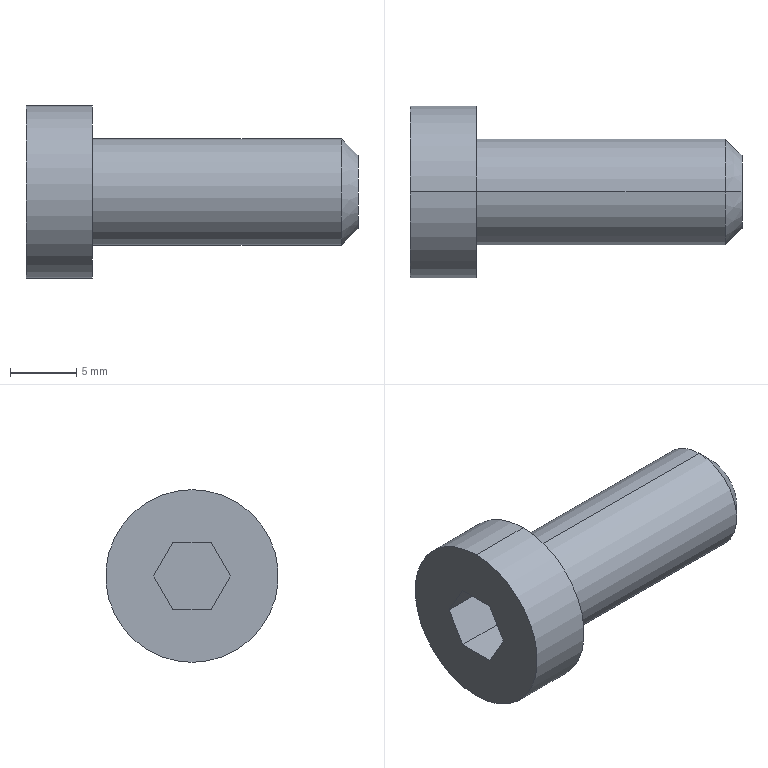Part | STEP file | CBSST8-20 | 1 solid | 16 faces | box 25 x 13 x 13 mm | volume 1569 mm3 | plane 10 | cylinder 4 | cone 2 | commonest cylinder face diameters 8 x2 13 x2
STEP:
#1=CARTESIAN_POINT('',(0.,0.,0.));
#2=DIRECTION('',(0.,0.,1.));
#3=DIRECTION('',(1.,0.,0.));
#4=AXIS2_PLACEMENT_3D('',#1,#2,#3);
#5=CARTESIAN_POINT('',(0.,0.,6.5));
#6=VERTEX_POINT('',#5);
#7=CARTESIAN_POINT('',(0.,0.,-6.5));
#8=VERTEX_POINT('',#7);
#9=CARTESIAN_POINT('',(0.,0.,0.));
#10=DIRECTION('',(-1.,0.,0.));
#11=DIRECTION('',(0.,0.,1.));
#12=AXIS2_PLACEMENT_3D('',#9,#10,#11);
#13=CIRCLE('',#12,6.5);
#14=CARTESIAN_POINT('',(-6.25,0.,0.));
#15=DIRECTION('',(-1.,0.,0.));
#16=DIRECTION('',(0.,0.,1.));
#17=AXIS2_PLACEMENT_3D('',#14,#15,#16);
#18=CYLINDRICAL_SURFACE('',#17,6.5);
#19=CARTESIAN_POINT('',(0.,-6.25));
#20=DIRECTION('',(1.,0.));
#21=VECTOR('',#20,1.);
#22=LINE('',#19,#21);
#23=(GEOMETRIC_REPRESENTATION_CONTEXT(2)PARAMETRIC_REPRESENTATION_CONTEXT()REPRESENTATION_CONTEXT('',''));
#24=DEFINITIONAL_REPRESENTATION('',(#22),#23);
#25=PCURVE('',#18,#24);
#26=CARTESIAN_POINT('',(0.,-4.4,0.));
#27=DIRECTION('',(1.,0.,0.));
#28=DIRECTION('',(0.,0.,-1.));
#29=AXIS2_PLACEMENT_3D('',#26,#27,#28);
#30=PLANE('',#29);
#31=CARTESIAN_POINT('',(-6.5,4.4));
#32=CARTESIAN_POINT('',(-6.5,15.658));
#33=CARTESIAN_POINT('',(3.25,10.029));
#34=CARTESIAN_POINT('',(13.,4.4));
#35=CARTESIAN_POINT('',(3.25,-1.229));
#36=CARTESIAN_POINT('',(-6.5,-6.858));
#37=CARTESIAN_POINT('',(-6.5,4.4));
#38=(BOUNDED_CURVE()B_SPLINE_CURVE(2,(#31,#32,#33,#34,#35,#36,#37),.UNSPECIFIED.,.T.,.F.)B_SPLINE_CURVE_WITH_KNOTS((1,2,2,2,2,1),(-2.094,0.,2.094,4.189,6.283,8.378),.UNSPECIFIED.)CURVE()GEOMETRIC_REPRESENTATION_ITEM()RATIONAL_B_SPLINE_CURVE((1.,0.5,1.,0.5,1.,0.5,1.))REPRESENTATION_ITEM(''));
#39=(GEOMETRIC_REPRESENTATION_CONTEXT(2)PARAMETRIC_REPRESENTATION_CONTEXT()REPRESENTATION_CONTEXT('',''));
#40=DEFINITIONAL_REPRESENTATION('',(#38),#39);
#41=PCURVE('',#30,#40);
#42=SURFACE_CURVE('',#13,(#25,#41),.PCURVE_S1.);
#43=EDGE_CURVE('',#6,#8,#42,.T.);
#44=ORIENTED_EDGE('',*,*,#43,.T.);
#45=CARTESIAN_POINT('',(-5.,0.,-6.5));
#46=VERTEX_POINT('',#45);
#47=CARTESIAN_POINT('',(-6.25,0.,-6.5));
#48=DIRECTION('',(-1.,0.,0.));
#49=VECTOR('',#48,1.);
#50=LINE('',#47,#49);
#51=CARTESIAN_POINT('',(3.142,0.));
#52=DIRECTION('',(0.,1.));
#53=VECTOR('',#52,1.);
#54=LINE('',#51,#53);
#55=(GEOMETRIC_REPRESENTATION_CONTEXT(2)PARAMETRIC_REPRESENTATION_CONTEXT()REPRESENTATION_CONTEXT('',''));
#56=DEFINITIONAL_REPRESENTATION('',(#54),#55);
#57=PCURVE('',#18,#56);
#58=CARTESIAN_POINT('',(-6.25,0.,0.));
#59=DIRECTION('',(-1.,0.,0.));
#60=DIRECTION('',(0.,0.,1.));
#61=AXIS2_PLACEMENT_3D('',#58,#59,#60);
#62=CYLINDRICAL_SURFACE('',#61,6.5);
#63=CARTESIAN_POINT('',(3.142,0.));
#64=DIRECTION('',(0.,1.));
#65=VECTOR('',#64,1.);
#66=LINE('',#63,#65);
#67=(GEOMETRIC_REPRESENTATION_CONTEXT(2)PARAMETRIC_REPRESENTATION_CONTEXT()REPRESENTATION_CONTEXT('',''));
#68=DEFINITIONAL_REPRESENTATION('',(#66),#67);
#69=PCURVE('',#62,#68);
#70=SURFACE_CURVE('',#50,(#57,#69),.PCURVE_S1.);
#71=EDGE_CURVE('',#8,#46,#70,.T.);
#72=ORIENTED_EDGE('',*,*,#71,.T.);
#73=CARTESIAN_POINT('',(-5.,0.,6.5));
#74=VERTEX_POINT('',#73);
#75=CARTESIAN_POINT('',(-5.,0.,0.));
#76=DIRECTION('',(-1.,0.,0.));
#77=DIRECTION('',(0.,0.,1.));
#78=AXIS2_PLACEMENT_3D('',#75,#76,#77);
#79=CIRCLE('',#78,6.5);
#80=CARTESIAN_POINT('',(0.,-1.25));
#81=DIRECTION('',(1.,0.));
#82=VECTOR('',#81,1.);
#83=LINE('',#80,#82);
#84=(GEOMETRIC_REPRESENTATION_CONTEXT(2)PARAMETRIC_REPRESENTATION_CONTEXT()REPRESENTATION_CONTEXT('',''));
#85=DEFINITIONAL_REPRESENTATION('',(#83),#84);
#86=PCURVE('',#18,#85);
#87=CARTESIAN_POINT('',(-5.,-6.5,0.));
#88=DIRECTION('',(-1.,0.,0.));
#89=DIRECTION('',(0.,0.,1.));
#90=AXIS2_PLACEMENT_3D('',#87,#88,#89);
#91=PLANE('',#90);
#92=CARTESIAN_POINT('',(0.,6.5));
#93=DIRECTION('',(1.,0.));
#94=AXIS2_PLACEMENT_2D('',#92,#93);
#95=CIRCLE('',#94,6.5);
#96=(GEOMETRIC_REPRESENTATION_CONTEXT(2)PARAMETRIC_REPRESENTATION_CONTEXT()REPRESENTATION_CONTEXT('',''));
#97=DEFINITIONAL_REPRESENTATION('',(#95),#96);
#98=PCURVE('',#91,#97);
#99=SURFACE_CURVE('',#79,(#86,#98),.PCURVE_S1.);
#100=EDGE_CURVE('',#74,#46,#99,.T.);
#101=ORIENTED_EDGE('',*,*,#100,.F.);
#102=CARTESIAN_POINT('',(-6.25,0.,6.5));
#103=DIRECTION('',(-1.,0.,0.));
#104=VECTOR('',#103,1.);
#105=LINE('',#102,#104);
#106=CARTESIAN_POINT('',(0.,0.));
#107=DIRECTION('',(0.,1.));
#108=VECTOR('',#107,1.);
#109=LINE('',#106,#108);
#110=(GEOMETRIC_REPRESENTATION_CONTEXT(2)PARAMETRIC_REPRESENTATION_CONTEXT()REPRESENTATION_CONTEXT('',''));
#111=DEFINITIONAL_REPRESENTATION('',(#109),#110);
#112=PCURVE('',#18,#111);
#113=CARTESIAN_POINT('',(6.283,0.));
#114=DIRECTION('',(0.,1.));
#115=VECTOR('',#114,1.);
#116=LINE('',#113,#115);
#117=(GEOMETRIC_REPRESENTATION_CONTEXT(2)PARAMETRIC_REPRESENTATION_CONTEXT()REPRESENTATION_CONTEXT('',''));
#118=DEFINITIONAL_REPRESENTATION('',(#116),#117);
#119=PCURVE('',#62,#118);
#120=SURFACE_CURVE('',#105,(#112,#119),.PCURVE_S1.);
#121=EDGE_CURVE('',#6,#74,#120,.T.);
#122=ORIENTED_EDGE('',*,*,#121,.F.);
#123=EDGE_LOOP('',(#44,#72,#101,#122));
#124=FACE_BOUND('',#123,.T.);
#125=ADVANCED_FACE('',(#124),#18,.T.);
#126=CARTESIAN_POINT('',(18.75,0.,4.));
#127=VERTEX_POINT('',#126);
#128=CARTESIAN_POINT('',(18.75,0.,-4.));
#129=VERTEX_POINT('',#128);
#130=CARTESIAN_POINT('',(18.75,0.,0.));
#131=DIRECTION('',(-1.,0.,0.));
#132=DIRECTION('',(0.,0.,1.));
#133=AXIS2_PLACEMENT_3D('',#130,#131,#132);
#134=CIRCLE('',#133,4.);
#135=CARTESIAN_POINT('',(-6.25,0.,0.));
#136=DIRECTION('',(-1.,0.,0.));
#137=DIRECTION('',(0.,0.,1.));
#138=AXIS2_PLACEMENT_3D('',#135,#136,#137);
#139=CYLINDRICAL_SURFACE('',#138,4.);
#140=CARTESIAN_POINT('',(0.,-25.));
#141=DIRECTION('',(1.,0.));
#142=VECTOR('',#141,1.);
#143=LINE('',#140,#142);
#144=(GEOMETRIC_REPRESENTATION_CONTEXT(2)PARAMETRIC_REPRESENTATION_CONTEXT()REPRESENTATION_CONTEXT('',''));
#145=DEFINITIONAL_REPRESENTATION('',(#143),#144);
#146=PCURVE('',#139,#145);
#147=CARTESIAN_POINT('',(18.75,0.,0.));
#148=DIRECTION('',(-1.,0.,0.));
#149=DIRECTION('',(0.,0.,1.));
#150=AXIS2_PLACEMENT_3D('',#147,#148,#149);
#151=CONICAL_SURFACE('',#150,4.,0.7854);
#152=CARTESIAN_POINT('',(0.,0.));
#153=DIRECTION('',(1.,0.));
#154=VECTOR('',#153,1.);
#155=LINE('',#152,#154);
#156=(GEOMETRIC_REPRESENTATION_CONTEXT(2)PARAMETRIC_REPRESENTATION_CONTEXT()REPRESENTATION_CONTEXT('',''));
#157=DEFINITIONAL_REPRESENTATION('',(#155),#156);
#158=PCURVE('',#151,#157);
#159=SURFACE_CURVE('',#134,(#146,#158),.PCURVE_S1.);
#160=EDGE_CURVE('',#127,#129,#159,.T.);
#161=ORIENTED_EDGE('',*,*,#160,.T.);
#162=CARTESIAN_POINT('',(0.,0.,-4.));
#163=VERTEX_POINT('',#162);
#164=CARTESIAN_POINT('',(-6.25,0.,-4.));
#165=DIRECTION('',(-1.,0.,0.));
#166=VECTOR('',#165,1.);
#167=LINE('',#164,#166);
#168=CARTESIAN_POINT('',(3.142,0.));
#169=DIRECTION('',(0.,1.));
#170=VECTOR('',#169,1.);
#171=LINE('',#168,#170);
#172=(GEOMETRIC_REPRESENTATION_CONTEXT(2)PARAMETRIC_REPRESENTATION_CONTEXT()REPRESENTATION_CONTEXT('',''));
#173=DEFINITIONAL_REPRESENTATION('',(#171),#172);
#174=PCURVE('',#139,#173);
#175=CARTESIAN_POINT('',(-6.25,0.,0.));
#176=DIRECTION('',(-1.,0.,0.));
#177=DIRECTION('',(0.,0.,1.));
#178=AXIS2_PLACEMENT_3D('',#175,#176,#177);
#179=CYLINDRICAL_SURFACE('',#178,4.);
#180=CARTESIAN_POINT('',(3.142,0.));
#181=DIRECTION('',(0.,1.));
#182=VECTOR('',#181,1.);
#183=LINE('',#180,#182);
#184=(GEOMETRIC_REPRESENTATION_CONTEXT(2)PARAMETRIC_REPRESENTATION_CONTEXT()REPRESENTATION_CONTEXT('',''));
#185=DEFINITIONAL_REPRESENTATION('',(#183),#184);
#186=PCURVE('',#179,#185);
#187=SURFACE_CURVE('',#167,(#174,#186),.PCURVE_S1.);
#188=EDGE_CURVE('',#129,#163,#187,.T.);
#189=ORIENTED_EDGE('',*,*,#188,.T.);
#190=CARTESIAN_POINT('',(0.,0.,4.));
#191=VERTEX_POINT('',#190);
#192=CARTESIAN_POINT('',(0.,0.,0.));
#193=DIRECTION('',(1.,0.,0.));
#194=DIRECTION('',(0.,0.,-1.));
#195=AXIS2_PLACEMENT_3D('',#192,#193,#194);
#196=CIRCLE('',#195,4.);
#197=CARTESIAN_POINT('',(3.142,-6.25));
#198=DIRECTION('',(-1.,0.));
#199=VECTOR('',#198,1.);
#200=LINE('',#197,#199);
#201=(GEOMETRIC_REPRESENTATION_CONTEXT(2)PARAMETRIC_REPRESENTATION_CONTEXT()REPRESENTATION_CONTEXT('',''));
#202=DEFINITIONAL_REPRESENTATION('',(#200),#201);
#203=PCURVE('',#139,#202);
#204=CARTESIAN_POINT('',(0.,4.4));
#205=DIRECTION('',(1.,0.));
#206=AXIS2_PLACEMENT_2D('',#204,#205);
#207=CIRCLE('',#206,4.);
#208=(GEOMETRIC_REPRESENTATION_CONTEXT(2)PARAMETRIC_REPRESENTATION_CONTEXT()REPRESENTATION_CONTEXT('',''));
#209=DEFINITIONAL_REPRESENTATION('',(#207),#208);
#210=PCURVE('',#30,#209);
#211=SURFACE_CURVE('',#196,(#203,#210),.PCURVE_S1.);
#212=EDGE_CURVE('',#163,#191,#211,.T.);
#213=ORIENTED_EDGE('',*,*,#212,.T.);
#214=CARTESIAN_POINT('',(-6.25,0.,4.));
#215=DIRECTION('',(-1.,0.,0.));
#216=VECTOR('',#215,1.);
#217=LINE('',#214,#216);
#218=CARTESIAN_POINT('',(0.,0.));
#219=DIRECTION('',(0.,1.));
#220=VECTOR('',#219,1.);
#221=LINE('',#218,#220);
#222=(GEOMETRIC_REPRESENTATION_CONTEXT(2)PARAMETRIC_REPRESENTATION_CONTEXT()REPRESENTATION_CONTEXT('',''));
#223=DEFINITIONAL_REPRESENTATION('',(#221),#222);
#224=PCURVE('',#139,#223);
#225=CARTESIAN_POINT('',(6.283,0.));
#226=DIRECTION('',(0.,1.));
#227=VECTOR('',#226,1.);
#228=LINE('',#225,#227);
#229=(GEOMETRIC_REPRESENTATION_CONTEXT(2)PARAMETRIC_REPRESENTATION_CONTEXT()REPRESENTATION_CONTEXT('',''));
#230=DEFINITIONAL_REPRESENTATION('',(#228),#229);
#231=PCURVE('',#179,#230);
#232=SURFACE_CURVE('',#217,(#224,#231),.PCURVE_S1.);
#233=EDGE_CURVE('',#127,#191,#232,.T.);
#234=ORIENTED_EDGE('',*,*,#233,.F.);
#235=EDGE_LOOP('',(#161,#189,#213,#234));
#236=FACE_BOUND('',#235,.T.);
#237=ADVANCED_FACE('',(#236),#139,.T.);
#238=CARTESIAN_POINT('',(20.,0.,2.75));
#239=VERTEX_POINT('',#238);
#240=CARTESIAN_POINT('',(20.,0.,-2.75));
#241=VERTEX_POINT('',#240);
#242=CARTESIAN_POINT('',(20.,0.,0.));
#243=DIRECTION('',(-1.,0.,0.));
#244=DIRECTION('',(0.,0.,1.));
#245=AXIS2_PLACEMENT_3D('',#242,#243,#244);
#246=CIRCLE('',#245,2.75);
#247=CARTESIAN_POINT('',(0.,-1.25));
#248=DIRECTION('',(1.,0.));
#249=VECTOR('',#248,1.);
#250=LINE('',#247,#249);
#251=(GEOMETRIC_REPRESENTATION_CONTEXT(2)PARAMETRIC_REPRESENTATION_CONTEXT()REPRESENTATION_CONTEXT('',''));
#252=DEFINITIONAL_REPRESENTATION('',(#250),#251);
#253=PCURVE('',#151,#252);
#254=CARTESIAN_POINT('',(20.,0.,0.));
#255=DIRECTION('',(1.,0.,0.));
#256=DIRECTION('',(0.,0.,-1.));
#257=AXIS2_PLACEMENT_3D('',#254,#255,#256);
#258=PLANE('',#257);
#259=CARTESIAN_POINT('',(-2.75,0.));
#260=CARTESIAN_POINT('',(-2.75,4.763));
#261=CARTESIAN_POINT('',(1.375,2.382));
#262=CARTESIAN_POINT('',(5.5,0.));
#263=CARTESIAN_POINT('',(1.375,-2.382));
#264=CARTESIAN_POINT('',(-2.75,-4.763));
#265=CARTESIAN_POINT('',(-2.75,0.));
#266=(BOUNDED_CURVE()B_SPLINE_CURVE(2,(#259,#260,#261,#262,#263,#264,#265),.UNSPECIFIED.,.T.,.F.)B_SPLINE_CURVE_WITH_KNOTS((1,2,2,2,2,1),(-2.094,0.,2.094,4.189,6.283,8.378),.UNSPECIFIED.)CURVE()GEOMETRIC_REPRESENTATION_ITEM()RATIONAL_B_SPLINE_CURVE((1.,0.5,1.,0.5,1.,0.5,1.))REPRESENTATION_ITEM(''));
#267=(GEOMETRIC_REPRESENTATION_CONTEXT(2)PARAMETRIC_REPRESENTATION_CONTEXT()REPRESENTATION_CONTEXT('',''));
#268=DEFINITIONAL_REPRESENTATION('',(#266),#267);
#269=PCURVE('',#258,#268);
#270=SURFACE_CURVE('',#246,(#253,#269),.PCURVE_S1.);
#271=EDGE_CURVE('',#239,#241,#270,.T.);
#272=ORIENTED_EDGE('',*,*,#271,.T.);
#273=CARTESIAN_POINT('',(18.75,0.,-4.));
#274=DIRECTION('',(-0.7071,0.,-0.7071));
#275=VECTOR('',#274,1.);
#276=LINE('',#273,#275);
#277=CARTESIAN_POINT('',(3.142,0.));
#278=DIRECTION('',(0.,1.));
#279=VECTOR('',#278,1.);
#280=LINE('',#277,#279);
#281=(GEOMETRIC_REPRESENTATION_CONTEXT(2)PARAMETRIC_REPRESENTATION_CONTEXT()REPRESENTATION_CONTEXT('',''));
#282=DEFINITIONAL_REPRESENTATION('',(#280),#281);
#283=PCURVE('',#151,#282);
#284=CARTESIAN_POINT('',(18.75,0.,0.));
#285=DIRECTION('',(-1.,0.,0.));
#286=DIRECTION('',(0.,0.,1.));
#287=AXIS2_PLACEMENT_3D('',#284,#285,#286);
#288=CONICAL_SURFACE('',#287,4.,0.7854);
#289=CARTESIAN_POINT('',(3.142,0.));
#290=DIRECTION('',(0.,1.));
#291=VECTOR('',#290,1.);
#292=LINE('',#289,#291);
#293=(GEOMETRIC_REPRESENTATION_CONTEXT(2)PARAMETRIC_REPRESENTATION_CONTEXT()REPRESENTATION_CONTEXT('',''));
#294=DEFINITIONAL_REPRESENTATION('',(#292),#293);
#295=PCURVE('',#288,#294);
#296=SURFACE_CURVE('',#276,(#283,#295),.PCURVE_S1.);
#297=EDGE_CURVE('',#241,#129,#296,.T.);
#298=ORIENTED_EDGE('',*,*,#297,.T.);
#299=ORIENTED_EDGE('',*,*,#160,.F.);
#300=CARTESIAN_POINT('',(18.75,0.,4.));
#301=DIRECTION('',(-0.7071,0.,0.7071));
#302=VECTOR('',#301,1.);
#303=LINE('',#300,#302);
#304=CARTESIAN_POINT('',(0.,0.));
#305=DIRECTION('',(0.,1.));
#306=VECTOR('',#305,1.);
#307=LINE('',#304,#306);
#308=(GEOMETRIC_REPRESENTATION_CONTEXT(2)PARAMETRIC_REPRESENTATION_CONTEXT()REPRESENTATION_CONTEXT('',''));
#309=DEFINITIONAL_REPRESENTATION('',(#307),#308);
#310=PCURVE('',#151,#309);
#311=CARTESIAN_POINT('',(6.283,0.));
#312=DIRECTION('',(0.,1.));
#313=VECTOR('',#312,1.);
#314=LINE('',#311,#313);
#315=(GEOMETRIC_REPRESENTATION_CONTEXT(2)PARAMETRIC_REPRESENTATION_CONTEXT()REPRESENTATION_CONTEXT('',''));
#316=DEFINITIONAL_REPRESENTATION('',(#314),#315);
#317=PCURVE('',#288,#316);
#318=SURFACE_CURVE('',#303,(#310,#317),.PCURVE_S1.);
#319=EDGE_CURVE('',#239,#127,#318,.T.);
#320=ORIENTED_EDGE('',*,*,#319,.F.);
#321=EDGE_LOOP('',(#272,#298,#299,#320));
#322=FACE_BOUND('',#321,.T.);
#323=ADVANCED_FACE('',(#322),#151,.T.);
#324=CARTESIAN_POINT('',(-5.,1.443,2.5));
#325=VERTEX_POINT('',#324);
#326=CARTESIAN_POINT('',(-5.,2.887,0.));
#327=VERTEX_POINT('',#326);
#328=CARTESIAN_POINT('',(-5.,1.443,2.5));
#329=DIRECTION('',(0.,0.5,-0.866));
#330=VECTOR('',#329,1.);
#331=LINE('',#328,#330);
#332=CARTESIAN_POINT('',(2.5,7.943));
#333=DIRECTION('',(-0.866,0.5));
#334=VECTOR('',#333,1.);
#335=LINE('',#332,#334);
#336=(GEOMETRIC_REPRESENTATION_CONTEXT(2)PARAMETRIC_REPRESENTATION_CONTEXT()REPRESENTATION_CONTEXT('',''));
#337=DEFINITIONAL_REPRESENTATION('',(#335),#336);
#338=PCURVE('',#91,#337);
#339=CARTESIAN_POINT('',(-1.2,1.443,2.5));
#340=DIRECTION('',(0.,0.866,0.5));
#341=DIRECTION('',(0.,-0.5,0.866));
#342=AXIS2_PLACEMENT_3D('',#339,#340,#341);
#343=PLANE('',#342);
#344=CARTESIAN_POINT('',(0.,-3.8));
#345=DIRECTION('',(-1.,0.));
#346=VECTOR('',#345,1.);
#347=LINE('',#344,#346);
#348=(GEOMETRIC_REPRESENTATION_CONTEXT(2)PARAMETRIC_REPRESENTATION_CONTEXT()REPRESENTATION_CONTEXT('',''));
#349=DEFINITIONAL_REPRESENTATION('',(#347),#348);
#350=PCURVE('',#343,#349);
#351=SURFACE_CURVE('',#331,(#338,#350),.PCURVE_S1.);
#352=EDGE_CURVE('',#325,#327,#351,.T.);
#353=ORIENTED_EDGE('',*,*,#352,.F.);
#354=CARTESIAN_POINT('',(-5.,-1.443,2.5));
#355=VERTEX_POINT('',#354);
#356=CARTESIAN_POINT('',(-5.,-1.443,2.5));
#357=DIRECTION('',(0.,1.,0.));
#358=VECTOR('',#357,1.);
#359=LINE('',#356,#358);
#360=CARTESIAN_POINT('',(2.5,5.057));
#361=DIRECTION('',(0.,1.));
#362=VECTOR('',#361,1.);
#363=LINE('',#360,#362);
#364=(GEOMETRIC_REPRESENTATION_CONTEXT(2)PARAMETRIC_REPRESENTATION_CONTEXT()REPRESENTATION_CONTEXT('',''));
#365=DEFINITIONAL_REPRESENTATION('',(#363),#364);
#366=PCURVE('',#91,#365);
#367=CARTESIAN_POINT('',(-1.2,-1.443,2.5));
#368=DIRECTION('',(0.,0.,1.));
#369=DIRECTION('',(1.,0.,0.));
#370=AXIS2_PLACEMENT_3D('',#367,#368,#369);
#371=PLANE('',#370);
#372=CARTESIAN_POINT('',(-3.8,0.));
#373=DIRECTION('',(0.,1.));
#374=VECTOR('',#373,1.);
#375=LINE('',#372,#374);
#376=(GEOMETRIC_REPRESENTATION_CONTEXT(2)PARAMETRIC_REPRESENTATION_CONTEXT()REPRESENTATION_CONTEXT('',''));
#377=DEFINITIONAL_REPRESENTATION('',(#375),#376);
#378=PCURVE('',#371,#377);
#379=SURFACE_CURVE('',#359,(#366,#378),.PCURVE_S1.);
#380=EDGE_CURVE('',#355,#325,#379,.T.);
#381=ORIENTED_EDGE('',*,*,#380,.F.);
#382=CARTESIAN_POINT('',(-5.,-2.887,0.));
#383=VERTEX_POINT('',#382);
#384=CARTESIAN_POINT('',(-5.,-2.887,0.));
#385=DIRECTION('',(0.,0.5,0.866));
#386=VECTOR('',#385,1.);
#387=LINE('',#384,#386);
#388=CARTESIAN_POINT('',(0.,3.613));
#389=DIRECTION('',(0.866,0.5));
#390=VECTOR('',#389,1.);
#391=LINE('',#388,#390);
#392=(GEOMETRIC_REPRESENTATION_CONTEXT(2)PARAMETRIC_REPRESENTATION_CONTEXT()REPRESENTATION_CONTEXT('',''));
#393=DEFINITIONAL_REPRESENTATION('',(#391),#392);
#394=PCURVE('',#91,#393);
#395=CARTESIAN_POINT('',(-1.2,-2.887,0.));
#396=DIRECTION('',(0.,-0.866,0.5));
#397=DIRECTION('',(0.,-0.5,-0.866));
#398=AXIS2_PLACEMENT_3D('',#395,#396,#397);
#399=PLANE('',#398);
#400=CARTESIAN_POINT('',(0.,-3.8));
#401=DIRECTION('',(-1.,0.));
#402=VECTOR('',#401,1.);
#403=LINE('',#400,#402);
#404=(GEOMETRIC_REPRESENTATION_CONTEXT(2)PARAMETRIC_REPRESENTATION_CONTEXT()REPRESENTATION_CONTEXT('',''));
#405=DEFINITIONAL_REPRESENTATION('',(#403),#404);
#406=PCURVE('',#399,#405);
#407=SURFACE_CURVE('',#387,(#394,#406),.PCURVE_S1.);
#408=EDGE_CURVE('',#383,#355,#407,.T.);
#409=ORIENTED_EDGE('',*,*,#408,.F.);
#410=CARTESIAN_POINT('',(-5.,-1.443,-2.5));
#411=VERTEX_POINT('',#410);
#412=CARTESIAN_POINT('',(-5.,-1.443,-2.5));
#413=DIRECTION('',(0.,-0.5,0.866));
#414=VECTOR('',#413,1.);
#415=LINE('',#412,#414);
#416=CARTESIAN_POINT('',(-2.5,5.057));
#417=DIRECTION('',(0.866,-0.5));
#418=VECTOR('',#417,1.);
#419=LINE('',#416,#418);
#420=(GEOMETRIC_REPRESENTATION_CONTEXT(2)PARAMETRIC_REPRESENTATION_CONTEXT()REPRESENTATION_CONTEXT('',''));
#421=DEFINITIONAL_REPRESENTATION('',(#419),#420);
#422=PCURVE('',#91,#421);
#423=CARTESIAN_POINT('',(-1.2,-1.443,-2.5));
#424=DIRECTION('',(0.,-0.866,-0.5));
#425=DIRECTION('',(0.,0.5,-0.866));
#426=AXIS2_PLACEMENT_3D('',#423,#424,#425);
#427=PLANE('',#426);
#428=CARTESIAN_POINT('',(0.,-3.8));
#429=DIRECTION('',(-1.,0.));
#430=VECTOR('',#429,1.);
#431=LINE('',#428,#430);
#432=(GEOMETRIC_REPRESENTATION_CONTEXT(2)PARAMETRIC_REPRESENTATION_CONTEXT()REPRESENTATION_CONTEXT('',''));
#433=DEFINITIONAL_REPRESENTATION('',(#431),#432);
#434=PCURVE('',#427,#433);
#435=SURFACE_CURVE('',#415,(#422,#434),.PCURVE_S1.);
#436=EDGE_CURVE('',#411,#383,#435,.T.);
#437=ORIENTED_EDGE('',*,*,#436,.F.);
#438=CARTESIAN_POINT('',(-5.,1.443,-2.5));
#439=VERTEX_POINT('',#438);
#440=CARTESIAN_POINT('',(-5.,1.443,-2.5));
#441=DIRECTION('',(0.,-1.,0.));
#442=VECTOR('',#441,1.);
#443=LINE('',#440,#442);
#444=CARTESIAN_POINT('',(-2.5,7.943));
#445=DIRECTION('',(0.,-1.));
#446=VECTOR('',#445,1.);
#447=LINE('',#444,#446);
#448=(GEOMETRIC_REPRESENTATION_CONTEXT(2)PARAMETRIC_REPRESENTATION_CONTEXT()REPRESENTATION_CONTEXT('',''));
#449=DEFINITIONAL_REPRESENTATION('',(#447),#448);
#450=PCURVE('',#91,#449);
#451=CARTESIAN_POINT('',(-1.2,1.443,-2.5));
#452=DIRECTION('',(0.,0.,-1.));
#453=DIRECTION('',(-1.,0.,0.));
#454=AXIS2_PLACEMENT_3D('',#451,#452,#453);
#455=PLANE('',#454);
#456=CARTESIAN_POINT('',(3.8,0.));
#457=DIRECTION('',(0.,-1.));
#458=VECTOR('',#457,1.);
#459=LINE('',#456,#458);
#460=(GEOMETRIC_REPRESENTATION_CONTEXT(2)PARAMETRIC_REPRESENTATION_CONTEXT()REPRESENTATION_CONTEXT('',''));
#461=DEFINITIONAL_REPRESENTATION('',(#459),#460);
#462=PCURVE('',#455,#461);
#463=SURFACE_CURVE('',#443,(#450,#462),.PCURVE_S1.);
#464=EDGE_CURVE('',#439,#411,#463,.T.);
#465=ORIENTED_EDGE('',*,*,#464,.F.);
#466=CARTESIAN_POINT('',(-5.,2.887,0.));
#467=DIRECTION('',(0.,-0.5,-0.866));
#468=VECTOR('',#467,1.);
#469=LINE('',#466,#468);
#470=CARTESIAN_POINT('',(0.,9.387));
#471=DIRECTION('',(-0.866,-0.5));
#472=VECTOR('',#471,1.);
#473=LINE('',#470,#472);
#474=(GEOMETRIC_REPRESENTATION_CONTEXT(2)PARAMETRIC_REPRESENTATION_CONTEXT()REPRESENTATION_CONTEXT('',''));
#475=DEFINITIONAL_REPRESENTATION('',(#473),#474);
#476=PCURVE('',#91,#475);
#477=CARTESIAN_POINT('',(-1.2,2.887,0.));
#478=DIRECTION('',(0.,0.866,-0.5));
#479=DIRECTION('',(0.,0.5,0.866));
#480=AXIS2_PLACEMENT_3D('',#477,#478,#479);
#481=PLANE('',#480);
#482=CARTESIAN_POINT('',(0.,-3.8));
#483=DIRECTION('',(-1.,0.));
#484=VECTOR('',#483,1.);
#485=LINE('',#482,#484);
#486=(GEOMETRIC_REPRESENTATION_CONTEXT(2)PARAMETRIC_REPRESENTATION_CONTEXT()REPRESENTATION_CONTEXT('',''));
#487=DEFINITIONAL_REPRESENTATION('',(#485),#486);
#488=PCURVE('',#481,#487);
#489=SURFACE_CURVE('',#469,(#476,#488),.PCURVE_S1.);
#490=EDGE_CURVE('',#327,#439,#489,.T.);
#491=ORIENTED_EDGE('',*,*,#490,.F.);
#492=EDGE_LOOP('',(#353,#381,#409,#437,#465,#491));
#493=FACE_BOUND('',#492,.T.);
#494=ORIENTED_EDGE('',*,*,#100,.T.);
#495=CARTESIAN_POINT('',(-5.,0.,0.));
#496=DIRECTION('',(-1.,0.,0.));
#497=DIRECTION('',(0.,0.,1.));
#498=AXIS2_PLACEMENT_3D('',#495,#496,#497);
#499=CIRCLE('',#498,6.5);
#500=CARTESIAN_POINT('',(0.,6.5));
#501=DIRECTION('',(1.,0.));
#502=AXIS2_PLACEMENT_2D('',#500,#501);
#503=CIRCLE('',#502,6.5);
#504=(GEOMETRIC_REPRESENTATION_CONTEXT(2)PARAMETRIC_REPRESENTATION_CONTEXT()REPRESENTATION_CONTEXT('',''));
#505=DEFINITIONAL_REPRESENTATION('',(#503),#504);
#506=PCURVE('',#91,#505);
#507=CARTESIAN_POINT('',(0.,-1.25));
#508=DIRECTION('',(1.,0.));
#509=VECTOR('',#508,1.);
#510=LINE('',#507,#509);
#511=(GEOMETRIC_REPRESENTATION_CONTEXT(2)PARAMETRIC_REPRESENTATION_CONTEXT()REPRESENTATION_CONTEXT('',''));
#512=DEFINITIONAL_REPRESENTATION('',(#510),#511);
#513=PCURVE('',#62,#512);
#514=SURFACE_CURVE('',#499,(#506,#513),.PCURVE_S1.);
#515=EDGE_CURVE('',#46,#74,#514,.T.);
#516=ORIENTED_EDGE('',*,*,#515,.T.);
#517=EDGE_LOOP('',(#494,#516));
#518=FACE_BOUND('',#517,.T.);
#519=ADVANCED_FACE('',(#493,#518),#91,.T.);
#520=ORIENTED_EDGE('',*,*,#271,.F.);
#521=CARTESIAN_POINT('',(20.,0.,0.));
#522=DIRECTION('',(-1.,0.,0.));
#523=DIRECTION('',(0.,0.,1.));
#524=AXIS2_PLACEMENT_3D('',#521,#522,#523);
#525=CIRCLE('',#524,2.75);
#526=CARTESIAN_POINT('',(-2.75,0.));
#527=CARTESIAN_POINT('',(-2.75,4.763));
#528=CARTESIAN_POINT('',(1.375,2.382));
#529=CARTESIAN_POINT('',(5.5,0.));
#530=CARTESIAN_POINT('',(1.375,-2.382));
#531=CARTESIAN_POINT('',(-2.75,-4.763));
#532=CARTESIAN_POINT('',(-2.75,0.));
#533=(BOUNDED_CURVE()B_SPLINE_CURVE(2,(#526,#527,#528,#529,#530,#531,#532),.UNSPECIFIED.,.T.,.F.)B_SPLINE_CURVE_WITH_KNOTS((1,2,2,2,2,1),(-2.094,0.,2.094,4.189,6.283,8.378),.UNSPECIFIED.)CURVE()GEOMETRIC_REPRESENTATION_ITEM()RATIONAL_B_SPLINE_CURVE((1.,0.5,1.,0.5,1.,0.5,1.))REPRESENTATION_ITEM(''));
#534=(GEOMETRIC_REPRESENTATION_CONTEXT(2)PARAMETRIC_REPRESENTATION_CONTEXT()REPRESENTATION_CONTEXT('',''));
#535=DEFINITIONAL_REPRESENTATION('',(#533),#534);
#536=PCURVE('',#258,#535);
#537=CARTESIAN_POINT('',(0.,-1.25));
#538=DIRECTION('',(1.,0.));
#539=VECTOR('',#538,1.);
#540=LINE('',#537,#539);
#541=(GEOMETRIC_REPRESENTATION_CONTEXT(2)PARAMETRIC_REPRESENTATION_CONTEXT()REPRESENTATION_CONTEXT('',''));
#542=DEFINITIONAL_REPRESENTATION('',(#540),#541);
#543=PCURVE('',#288,#542);
#544=SURFACE_CURVE('',#525,(#536,#543),.PCURVE_S1.);
#545=EDGE_CURVE('',#241,#239,#544,.T.);
#546=ORIENTED_EDGE('',*,*,#545,.F.);
#547=EDGE_LOOP('',(#520,#546));
#548=FACE_BOUND('',#547,.T.);
#549=ADVANCED_FACE('',(#548),#258,.T.);
#550=ORIENTED_EDGE('',*,*,#297,.F.);
#551=ORIENTED_EDGE('',*,*,#545,.T.);
#552=ORIENTED_EDGE('',*,*,#319,.T.);
#553=CARTESIAN_POINT('',(18.75,0.,0.));
#554=DIRECTION('',(-1.,0.,0.));
#555=DIRECTION('',(0.,0.,1.));
#556=AXIS2_PLACEMENT_3D('',#553,#554,#555);
#557=CIRCLE('',#556,4.);
#558=CARTESIAN_POINT('',(0.,0.));
#559=DIRECTION('',(1.,0.));
#560=VECTOR('',#559,1.);
#561=LINE('',#558,#560);
#562=(GEOMETRIC_REPRESENTATION_CONTEXT(2)PARAMETRIC_REPRESENTATION_CONTEXT()REPRESENTATION_CONTEXT('',''));
#563=DEFINITIONAL_REPRESENTATION('',(#561),#562);
#564=PCURVE('',#288,#563);
#565=CARTESIAN_POINT('',(0.,-25.));
#566=DIRECTION('',(1.,0.));
#567=VECTOR('',#566,1.);
#568=LINE('',#565,#567);
#569=(GEOMETRIC_REPRESENTATION_CONTEXT(2)PARAMETRIC_REPRESENTATION_CONTEXT()REPRESENTATION_CONTEXT('',''));
#570=DEFINITIONAL_REPRESENTATION('',(#568),#569);
#571=PCURVE('',#179,#570);
#572=SURFACE_CURVE('',#557,(#564,#571),.PCURVE_S1.);
#573=EDGE_CURVE('',#129,#127,#572,.T.);
#574=ORIENTED_EDGE('',*,*,#573,.F.);
#575=EDGE_LOOP('',(#550,#551,#552,#574));
#576=FACE_BOUND('',#575,.T.);
#577=ADVANCED_FACE('',(#576),#288,.T.);
#578=ORIENTED_EDGE('',*,*,#188,.F.);
#579=ORIENTED_EDGE('',*,*,#573,.T.);
#580=ORIENTED_EDGE('',*,*,#233,.T.);
#581=CARTESIAN_POINT('',(0.,0.,0.));
#582=DIRECTION('',(1.,0.,0.));
#583=DIRECTION('',(0.,0.,-1.));
#584=AXIS2_PLACEMENT_3D('',#581,#582,#583);
#585=CIRCLE('',#584,4.);
#586=CARTESIAN_POINT('',(9.425,-6.25));
#587=DIRECTION('',(-1.,0.));
#588=VECTOR('',#587,1.);
#589=LINE('',#586,#588);
#590=(GEOMETRIC_REPRESENTATION_CONTEXT(2)PARAMETRIC_REPRESENTATION_CONTEXT()REPRESENTATION_CONTEXT('',''));
#591=DEFINITIONAL_REPRESENTATION('',(#589),#590);
#592=PCURVE('',#179,#591);
#593=CARTESIAN_POINT('',(0.,4.4));
#594=DIRECTION('',(1.,0.));
#595=AXIS2_PLACEMENT_2D('',#593,#594);
#596=CIRCLE('',#595,4.);
#597=(GEOMETRIC_REPRESENTATION_CONTEXT(2)PARAMETRIC_REPRESENTATION_CONTEXT()REPRESENTATION_CONTEXT('',''));
#598=DEFINITIONAL_REPRESENTATION('',(#596),#597);
#599=PCURVE('',#30,#598);
#600=SURFACE_CURVE('',#585,(#592,#599),.PCURVE_S1.);
#601=EDGE_CURVE('',#191,#163,#600,.T.);
#602=ORIENTED_EDGE('',*,*,#601,.T.);
#603=EDGE_LOOP('',(#578,#579,#580,#602));
#604=FACE_BOUND('',#603,.T.);
#605=ADVANCED_FACE('',(#604),#179,.T.);
#606=ORIENTED_EDGE('',*,*,#43,.F.);
#607=CARTESIAN_POINT('',(0.,0.,0.));
#608=DIRECTION('',(-1.,0.,0.));
#609=DIRECTION('',(0.,0.,1.));
#610=AXIS2_PLACEMENT_3D('',#607,#608,#609);
#611=CIRCLE('',#610,6.5);
#612=CARTESIAN_POINT('',(-6.5,4.4));
#613=CARTESIAN_POINT('',(-6.5,15.658));
#614=CARTESIAN_POINT('',(3.25,10.029));
#615=CARTESIAN_POINT('',(13.,4.4));
#616=CARTESIAN_POINT('',(3.25,-1.229));
#617=CARTESIAN_POINT('',(-6.5,-6.858));
#618=CARTESIAN_POINT('',(-6.5,4.4));
#619=(BOUNDED_CURVE()B_SPLINE_CURVE(2,(#612,#613,#614,#615,#616,#617,#618),.UNSPECIFIED.,.T.,.F.)B_SPLINE_CURVE_WITH_KNOTS((1,2,2,2,2,1),(-2.094,0.,2.094,4.189,6.283,8.378),.UNSPECIFIED.)CURVE()GEOMETRIC_REPRESENTATION_ITEM()RATIONAL_B_SPLINE_CURVE((1.,0.5,1.,0.5,1.,0.5,1.))REPRESENTATION_ITEM(''));
#620=(GEOMETRIC_REPRESENTATION_CONTEXT(2)PARAMETRIC_REPRESENTATION_CONTEXT()REPRESENTATION_CONTEXT('',''));
#621=DEFINITIONAL_REPRESENTATION('',(#619),#620);
#622=PCURVE('',#30,#621);
#623=CARTESIAN_POINT('',(0.,-6.25));
#624=DIRECTION('',(1.,0.));
#625=VECTOR('',#624,1.);
#626=LINE('',#623,#625);
#627=(GEOMETRIC_REPRESENTATION_CONTEXT(2)PARAMETRIC_REPRESENTATION_CONTEXT()REPRESENTATION_CONTEXT('',''));
#628=DEFINITIONAL_REPRESENTATION('',(#626),#627);
#629=PCURVE('',#62,#628);
#630=SURFACE_CURVE('',#611,(#622,#629),.PCURVE_S1.);
#631=EDGE_CURVE('',#8,#6,#630,.T.);
#632=ORIENTED_EDGE('',*,*,#631,.F.);
#633=EDGE_LOOP('',(#606,#632));
#634=FACE_BOUND('',#633,.T.);
#635=ORIENTED_EDGE('',*,*,#601,.F.);
#636=ORIENTED_EDGE('',*,*,#212,.F.);
#637=EDGE_LOOP('',(#635,#636));
#638=FACE_BOUND('',#637,.T.);
#639=ADVANCED_FACE('',(#634,#638),#30,.T.);
#640=ORIENTED_EDGE('',*,*,#71,.F.);
#641=ORIENTED_EDGE('',*,*,#631,.T.);
#642=ORIENTED_EDGE('',*,*,#121,.T.);
#643=ORIENTED_EDGE('',*,*,#515,.F.);
#644=EDGE_LOOP('',(#640,#641,#642,#643));
#645=FACE_BOUND('',#644,.T.);
#646=ADVANCED_FACE('',(#645),#62,.T.);
#647=ORIENTED_EDGE('',*,*,#352,.T.);
#648=CARTESIAN_POINT('',(-1.2,2.887,0.));
#649=VERTEX_POINT('',#648);
#650=CARTESIAN_POINT('',(-1.2,2.887,0.));
#651=DIRECTION('',(-1.,0.,0.));
#652=VECTOR('',#651,1.);
#653=LINE('',#650,#652);
#654=CARTESIAN_POINT('',(-2.887,0.));
#655=DIRECTION('',(0.,-1.));
#656=VECTOR('',#655,1.);
#657=LINE('',#654,#656);
#658=(GEOMETRIC_REPRESENTATION_CONTEXT(2)PARAMETRIC_REPRESENTATION_CONTEXT()REPRESENTATION_CONTEXT('',''));
#659=DEFINITIONAL_REPRESENTATION('',(#657),#658);
#660=PCURVE('',#343,#659);
#661=CARTESIAN_POINT('',(0.,0.));
#662=DIRECTION('',(0.,-1.));
#663=VECTOR('',#662,1.);
#664=LINE('',#661,#663);
#665=(GEOMETRIC_REPRESENTATION_CONTEXT(2)PARAMETRIC_REPRESENTATION_CONTEXT()REPRESENTATION_CONTEXT('',''));
#666=DEFINITIONAL_REPRESENTATION('',(#664),#665);
#667=PCURVE('',#481,#666);
#668=SURFACE_CURVE('',#653,(#660,#667),.PCURVE_S1.);
#669=EDGE_CURVE('',#649,#327,#668,.T.);
#670=ORIENTED_EDGE('',*,*,#669,.F.);
#671=CARTESIAN_POINT('',(-1.2,1.443,2.5));
#672=VERTEX_POINT('',#671);
#673=CARTESIAN_POINT('',(-1.2,1.443,2.5));
#674=DIRECTION('',(0.,0.5,-0.866));
#675=VECTOR('',#674,1.);
#676=LINE('',#673,#675);
#677=CARTESIAN_POINT('',(0.,0.));
#678=DIRECTION('',(-1.,0.));
#679=VECTOR('',#678,1.);
#680=LINE('',#677,#679);
#681=(GEOMETRIC_REPRESENTATION_CONTEXT(2)PARAMETRIC_REPRESENTATION_CONTEXT()REPRESENTATION_CONTEXT('',''));
#682=DEFINITIONAL_REPRESENTATION('',(#680),#681);
#683=PCURVE('',#343,#682);
#684=CARTESIAN_POINT('',(-1.2,0.,0.));
#685=DIRECTION('',(-1.,0.,0.));
#686=DIRECTION('',(0.,0.,1.));
#687=AXIS2_PLACEMENT_3D('',#684,#685,#686);
#688=PLANE('',#687);
#689=CARTESIAN_POINT('',(2.5,1.443));
#690=DIRECTION('',(-0.866,0.5));
#691=VECTOR('',#690,1.);
#692=LINE('',#689,#691);
#693=(GEOMETRIC_REPRESENTATION_CONTEXT(2)PARAMETRIC_REPRESENTATION_CONTEXT()REPRESENTATION_CONTEXT('',''));
#694=DEFINITIONAL_REPRESENTATION('',(#692),#693);
#695=PCURVE('',#688,#694);
#696=SURFACE_CURVE('',#676,(#683,#695),.PCURVE_S1.);
#697=EDGE_CURVE('',#672,#649,#696,.T.);
#698=ORIENTED_EDGE('',*,*,#697,.F.);
#699=CARTESIAN_POINT('',(-1.2,1.443,2.5));
#700=DIRECTION('',(-1.,0.,0.));
#701=VECTOR('',#700,1.);
#702=LINE('',#699,#701);
#703=CARTESIAN_POINT('',(0.,0.));
#704=DIRECTION('',(0.,-1.));
#705=VECTOR('',#704,1.);
#706=LINE('',#703,#705);
#707=(GEOMETRIC_REPRESENTATION_CONTEXT(2)PARAMETRIC_REPRESENTATION_CONTEXT()REPRESENTATION_CONTEXT('',''));
#708=DEFINITIONAL_REPRESENTATION('',(#706),#707);
#709=PCURVE('',#343,#708);
#710=CARTESIAN_POINT('',(0.,2.887));
#711=DIRECTION('',(-1.,0.));
#712=VECTOR('',#711,1.);
#713=LINE('',#710,#712);
#714=(GEOMETRIC_REPRESENTATION_CONTEXT(2)PARAMETRIC_REPRESENTATION_CONTEXT()REPRESENTATION_CONTEXT('',''));
#715=DEFINITIONAL_REPRESENTATION('',(#713),#714);
#716=PCURVE('',#371,#715);
#717=SURFACE_CURVE('',#702,(#709,#716),.PCURVE_S1.);
#718=EDGE_CURVE('',#672,#325,#717,.T.);
#719=ORIENTED_EDGE('',*,*,#718,.T.);
#720=EDGE_LOOP('',(#647,#670,#698,#719));
#721=FACE_BOUND('',#720,.T.);
#722=ADVANCED_FACE('',(#721),#343,.F.);
#723=ORIENTED_EDGE('',*,*,#380,.T.);
#724=ORIENTED_EDGE('',*,*,#718,.F.);
#725=CARTESIAN_POINT('',(-1.2,-1.443,2.5));
#726=VERTEX_POINT('',#725);
#727=CARTESIAN_POINT('',(-1.2,-1.443,2.5));
#728=DIRECTION('',(0.,1.,0.));
#729=VECTOR('',#728,1.);
#730=LINE('',#727,#729);
#731=CARTESIAN_POINT('',(0.,0.));
#732=DIRECTION('',(0.,1.));
#733=VECTOR('',#732,1.);
#734=LINE('',#731,#733);
#735=(GEOMETRIC_REPRESENTATION_CONTEXT(2)PARAMETRIC_REPRESENTATION_CONTEXT()REPRESENTATION_CONTEXT('',''));
#736=DEFINITIONAL_REPRESENTATION('',(#734),#735);
#737=PCURVE('',#371,#736);
#738=CARTESIAN_POINT('',(2.5,-1.443));
#739=DIRECTION('',(0.,1.));
#740=VECTOR('',#739,1.);
#741=LINE('',#738,#740);
#742=(GEOMETRIC_REPRESENTATION_CONTEXT(2)PARAMETRIC_REPRESENTATION_CONTEXT()REPRESENTATION_CONTEXT('',''));
#743=DEFINITIONAL_REPRESENTATION('',(#741),#742);
#744=PCURVE('',#688,#743);
#745=SURFACE_CURVE('',#730,(#737,#744),.PCURVE_S1.);
#746=EDGE_CURVE('',#726,#672,#745,.T.);
#747=ORIENTED_EDGE('',*,*,#746,.F.);
#748=CARTESIAN_POINT('',(-1.2,-1.443,2.5));
#749=DIRECTION('',(-1.,0.,0.));
#750=VECTOR('',#749,1.);
#751=LINE('',#748,#750);
#752=CARTESIAN_POINT('',(0.,0.));
#753=DIRECTION('',(-1.,0.));
#754=VECTOR('',#753,1.);
#755=LINE('',#752,#754);
#756=(GEOMETRIC_REPRESENTATION_CONTEXT(2)PARAMETRIC_REPRESENTATION_CONTEXT()REPRESENTATION_CONTEXT('',''));
#757=DEFINITIONAL_REPRESENTATION('',(#755),#756);
#758=PCURVE('',#371,#757);
#759=CARTESIAN_POINT('',(-2.887,0.));
#760=DIRECTION('',(0.,-1.));
#761=VECTOR('',#760,1.);
#762=LINE('',#759,#761);
#763=(GEOMETRIC_REPRESENTATION_CONTEXT(2)PARAMETRIC_REPRESENTATION_CONTEXT()REPRESENTATION_CONTEXT('',''));
#764=DEFINITIONAL_REPRESENTATION('',(#762),#763);
#765=PCURVE('',#399,#764);
#766=SURFACE_CURVE('',#751,(#758,#765),.PCURVE_S1.);
#767=EDGE_CURVE('',#726,#355,#766,.T.);
#768=ORIENTED_EDGE('',*,*,#767,.T.);
#769=EDGE_LOOP('',(#723,#724,#747,#768));
#770=FACE_BOUND('',#769,.T.);
#771=ADVANCED_FACE('',(#770),#371,.F.);
#772=ORIENTED_EDGE('',*,*,#408,.T.);
#773=ORIENTED_EDGE('',*,*,#767,.F.);
#774=CARTESIAN_POINT('',(-1.2,-2.887,0.));
#775=VERTEX_POINT('',#774);
#776=CARTESIAN_POINT('',(-1.2,-2.887,0.));
#777=DIRECTION('',(0.,0.5,0.866));
#778=VECTOR('',#777,1.);
#779=LINE('',#776,#778);
#780=CARTESIAN_POINT('',(0.,0.));
#781=DIRECTION('',(-1.,0.));
#782=VECTOR('',#781,1.);
#783=LINE('',#780,#782);
#784=(GEOMETRIC_REPRESENTATION_CONTEXT(2)PARAMETRIC_REPRESENTATION_CONTEXT()REPRESENTATION_CONTEXT('',''));
#785=DEFINITIONAL_REPRESENTATION('',(#783),#784);
#786=PCURVE('',#399,#785);
#787=CARTESIAN_POINT('',(0.,-2.887));
#788=DIRECTION('',(0.866,0.5));
#789=VECTOR('',#788,1.);
#790=LINE('',#787,#789);
#791=(GEOMETRIC_REPRESENTATION_CONTEXT(2)PARAMETRIC_REPRESENTATION_CONTEXT()REPRESENTATION_CONTEXT('',''));
#792=DEFINITIONAL_REPRESENTATION('',(#790),#791);
#793=PCURVE('',#688,#792);
#794=SURFACE_CURVE('',#779,(#786,#793),.PCURVE_S1.);
#795=EDGE_CURVE('',#775,#726,#794,.T.);
#796=ORIENTED_EDGE('',*,*,#795,.F.);
#797=CARTESIAN_POINT('',(-1.2,-2.887,0.));
#798=DIRECTION('',(-1.,0.,0.));
#799=VECTOR('',#798,1.);
#800=LINE('',#797,#799);
#801=CARTESIAN_POINT('',(0.,0.));
#802=DIRECTION('',(0.,-1.));
#803=VECTOR('',#802,1.);
#804=LINE('',#801,#803);
#805=(GEOMETRIC_REPRESENTATION_CONTEXT(2)PARAMETRIC_REPRESENTATION_CONTEXT()REPRESENTATION_CONTEXT('',''));
#806=DEFINITIONAL_REPRESENTATION('',(#804),#805);
#807=PCURVE('',#399,#806);
#808=CARTESIAN_POINT('',(-2.887,0.));
#809=DIRECTION('',(0.,-1.));
#810=VECTOR('',#809,1.);
#811=LINE('',#808,#810);
#812=(GEOMETRIC_REPRESENTATION_CONTEXT(2)PARAMETRIC_REPRESENTATION_CONTEXT()REPRESENTATION_CONTEXT('',''));
#813=DEFINITIONAL_REPRESENTATION('',(#811),#812);
#814=PCURVE('',#427,#813);
#815=SURFACE_CURVE('',#800,(#807,#814),.PCURVE_S1.);
#816=EDGE_CURVE('',#775,#383,#815,.T.);
#817=ORIENTED_EDGE('',*,*,#816,.T.);
#818=EDGE_LOOP('',(#772,#773,#796,#817));
#819=FACE_BOUND('',#818,.T.);
#820=ADVANCED_FACE('',(#819),#399,.F.);
#821=ORIENTED_EDGE('',*,*,#436,.T.);
#822=ORIENTED_EDGE('',*,*,#816,.F.);
#823=CARTESIAN_POINT('',(-1.2,-1.443,-2.5));
#824=VERTEX_POINT('',#823);
#825=CARTESIAN_POINT('',(-1.2,-1.443,-2.5));
#826=DIRECTION('',(0.,-0.5,0.866));
#827=VECTOR('',#826,1.);
#828=LINE('',#825,#827);
#829=CARTESIAN_POINT('',(0.,0.));
#830=DIRECTION('',(-1.,0.));
#831=VECTOR('',#830,1.);
#832=LINE('',#829,#831);
#833=(GEOMETRIC_REPRESENTATION_CONTEXT(2)PARAMETRIC_REPRESENTATION_CONTEXT()REPRESENTATION_CONTEXT('',''));
#834=DEFINITIONAL_REPRESENTATION('',(#832),#833);
#835=PCURVE('',#427,#834);
#836=CARTESIAN_POINT('',(-2.5,-1.443));
#837=DIRECTION('',(0.866,-0.5));
#838=VECTOR('',#837,1.);
#839=LINE('',#836,#838);
#840=(GEOMETRIC_REPRESENTATION_CONTEXT(2)PARAMETRIC_REPRESENTATION_CONTEXT()REPRESENTATION_CONTEXT('',''));
#841=DEFINITIONAL_REPRESENTATION('',(#839),#840);
#842=PCURVE('',#688,#841);
#843=SURFACE_CURVE('',#828,(#835,#842),.PCURVE_S1.);
#844=EDGE_CURVE('',#824,#775,#843,.T.);
#845=ORIENTED_EDGE('',*,*,#844,.F.);
#846=CARTESIAN_POINT('',(-1.2,-1.443,-2.5));
#847=DIRECTION('',(-1.,0.,0.));
#848=VECTOR('',#847,1.);
#849=LINE('',#846,#848);
#850=CARTESIAN_POINT('',(0.,0.));
#851=DIRECTION('',(0.,-1.));
#852=VECTOR('',#851,1.);
#853=LINE('',#850,#852);
#854=(GEOMETRIC_REPRESENTATION_CONTEXT(2)PARAMETRIC_REPRESENTATION_CONTEXT()REPRESENTATION_CONTEXT('',''));
#855=DEFINITIONAL_REPRESENTATION('',(#853),#854);
#856=PCURVE('',#427,#855);
#857=CARTESIAN_POINT('',(0.,-2.887));
#858=DIRECTION('',(1.,0.));
#859=VECTOR('',#858,1.);
#860=LINE('',#857,#859);
#861=(GEOMETRIC_REPRESENTATION_CONTEXT(2)PARAMETRIC_REPRESENTATION_CONTEXT()REPRESENTATION_CONTEXT('',''));
#862=DEFINITIONAL_REPRESENTATION('',(#860),#861);
#863=PCURVE('',#455,#862);
#864=SURFACE_CURVE('',#849,(#856,#863),.PCURVE_S1.);
#865=EDGE_CURVE('',#824,#411,#864,.T.);
#866=ORIENTED_EDGE('',*,*,#865,.T.);
#867=EDGE_LOOP('',(#821,#822,#845,#866));
#868=FACE_BOUND('',#867,.T.);
#869=ADVANCED_FACE('',(#868),#427,.F.);
#870=ORIENTED_EDGE('',*,*,#464,.T.);
#871=ORIENTED_EDGE('',*,*,#865,.F.);
#872=CARTESIAN_POINT('',(-1.2,1.443,-2.5));
#873=VERTEX_POINT('',#872);
#874=CARTESIAN_POINT('',(-1.2,1.443,-2.5));
#875=DIRECTION('',(0.,-1.,0.));
#876=VECTOR('',#875,1.);
#877=LINE('',#874,#876);
#878=CARTESIAN_POINT('',(0.,0.));
#879=DIRECTION('',(0.,-1.));
#880=VECTOR('',#879,1.);
#881=LINE('',#878,#880);
#882=(GEOMETRIC_REPRESENTATION_CONTEXT(2)PARAMETRIC_REPRESENTATION_CONTEXT()REPRESENTATION_CONTEXT('',''));
#883=DEFINITIONAL_REPRESENTATION('',(#881),#882);
#884=PCURVE('',#455,#883);
#885=CARTESIAN_POINT('',(-2.5,1.443));
#886=DIRECTION('',(0.,-1.));
#887=VECTOR('',#886,1.);
#888=LINE('',#885,#887);
#889=(GEOMETRIC_REPRESENTATION_CONTEXT(2)PARAMETRIC_REPRESENTATION_CONTEXT()REPRESENTATION_CONTEXT('',''));
#890=DEFINITIONAL_REPRESENTATION('',(#888),#889);
#891=PCURVE('',#688,#890);
#892=SURFACE_CURVE('',#877,(#884,#891),.PCURVE_S1.);
#893=EDGE_CURVE('',#873,#824,#892,.T.);
#894=ORIENTED_EDGE('',*,*,#893,.F.);
#895=CARTESIAN_POINT('',(-1.2,1.443,-2.5));
#896=DIRECTION('',(-1.,0.,0.));
#897=VECTOR('',#896,1.);
#898=LINE('',#895,#897);
#899=CARTESIAN_POINT('',(0.,0.));
#900=DIRECTION('',(1.,0.));
#901=VECTOR('',#900,1.);
#902=LINE('',#899,#901);
#903=(GEOMETRIC_REPRESENTATION_CONTEXT(2)PARAMETRIC_REPRESENTATION_CONTEXT()REPRESENTATION_CONTEXT('',''));
#904=DEFINITIONAL_REPRESENTATION('',(#902),#903);
#905=PCURVE('',#455,#904);
#906=CARTESIAN_POINT('',(-2.887,0.));
#907=DIRECTION('',(0.,-1.));
#908=VECTOR('',#907,1.);
#909=LINE('',#906,#908);
#910=(GEOMETRIC_REPRESENTATION_CONTEXT(2)PARAMETRIC_REPRESENTATION_CONTEXT()REPRESENTATION_CONTEXT('',''));
#911=DEFINITIONAL_REPRESENTATION('',(#909),#910);
#912=PCURVE('',#481,#911);
#913=SURFACE_CURVE('',#898,(#905,#912),.PCURVE_S1.);
#914=EDGE_CURVE('',#873,#439,#913,.T.);
#915=ORIENTED_EDGE('',*,*,#914,.T.);
#916=EDGE_LOOP('',(#870,#871,#894,#915));
#917=FACE_BOUND('',#916,.T.);
#918=ADVANCED_FACE('',(#917),#455,.F.);
#919=ORIENTED_EDGE('',*,*,#490,.T.);
#920=ORIENTED_EDGE('',*,*,#914,.F.);
#921=CARTESIAN_POINT('',(-1.2,2.887,0.));
#922=DIRECTION('',(0.,-0.5,-0.866));
#923=VECTOR('',#922,1.);
#924=LINE('',#921,#923);
#925=CARTESIAN_POINT('',(0.,0.));
#926=DIRECTION('',(-1.,0.));
#927=VECTOR('',#926,1.);
#928=LINE('',#925,#927);
#929=(GEOMETRIC_REPRESENTATION_CONTEXT(2)PARAMETRIC_REPRESENTATION_CONTEXT()REPRESENTATION_CONTEXT('',''));
#930=DEFINITIONAL_REPRESENTATION('',(#928),#929);
#931=PCURVE('',#481,#930);
#932=CARTESIAN_POINT('',(0.,2.887));
#933=DIRECTION('',(-0.866,-0.5));
#934=VECTOR('',#933,1.);
#935=LINE('',#932,#934);
#936=(GEOMETRIC_REPRESENTATION_CONTEXT(2)PARAMETRIC_REPRESENTATION_CONTEXT()REPRESENTATION_CONTEXT('',''));
#937=DEFINITIONAL_REPRESENTATION('',(#935),#936);
#938=PCURVE('',#688,#937);
#939=SURFACE_CURVE('',#924,(#931,#938),.PCURVE_S1.);
#940=EDGE_CURVE('',#649,#873,#939,.T.);
#941=ORIENTED_EDGE('',*,*,#940,.F.);
#942=ORIENTED_EDGE('',*,*,#669,.T.);
#943=EDGE_LOOP('',(#919,#920,#941,#942));
#944=FACE_BOUND('',#943,.T.);
#945=ADVANCED_FACE('',(#944),#481,.F.);
#946=ORIENTED_EDGE('',*,*,#697,.T.);
#947=ORIENTED_EDGE('',*,*,#940,.T.);
#948=ORIENTED_EDGE('',*,*,#893,.T.);
#949=ORIENTED_EDGE('',*,*,#844,.T.);
#950=ORIENTED_EDGE('',*,*,#795,.T.);
#951=ORIENTED_EDGE('',*,*,#746,.T.);
#952=EDGE_LOOP('',(#946,#947,#948,#949,#950,#951));
#953=FACE_BOUND('',#952,.T.);
#954=ADVANCED_FACE('',(#953),#688,.T.);
#955=CLOSED_SHELL('',(#125,#237,#323,#519,#549,#577,#605,#639,#646,#722,#771,#820,#869,#918,#945,#954));
#956=MANIFOLD_SOLID_BREP('',#955);
#957=(LENGTH_UNIT()NAMED_UNIT(*)SI_UNIT(.MILLI.,.METRE.));
#958=UNCERTAINTY_MEASURE_WITH_UNIT(LENGTH_MEASURE(0.0000001),#957,'','');
#959=(NAMED_UNIT(*)PLANE_ANGLE_UNIT()SI_UNIT($,.RADIAN.));
#960=(NAMED_UNIT(*)SI_UNIT($,.STERADIAN.)SOLID_ANGLE_UNIT());
#961=(GEOMETRIC_REPRESENTATION_CONTEXT(3)GLOBAL_UNCERTAINTY_ASSIGNED_CONTEXT((#958))GLOBAL_UNIT_ASSIGNED_CONTEXT((#957,#959,#960))REPRESENTATION_CONTEXT('',''));
#962=ADVANCED_BREP_SHAPE_REPRESENTATION('',(#4,#956),#961);